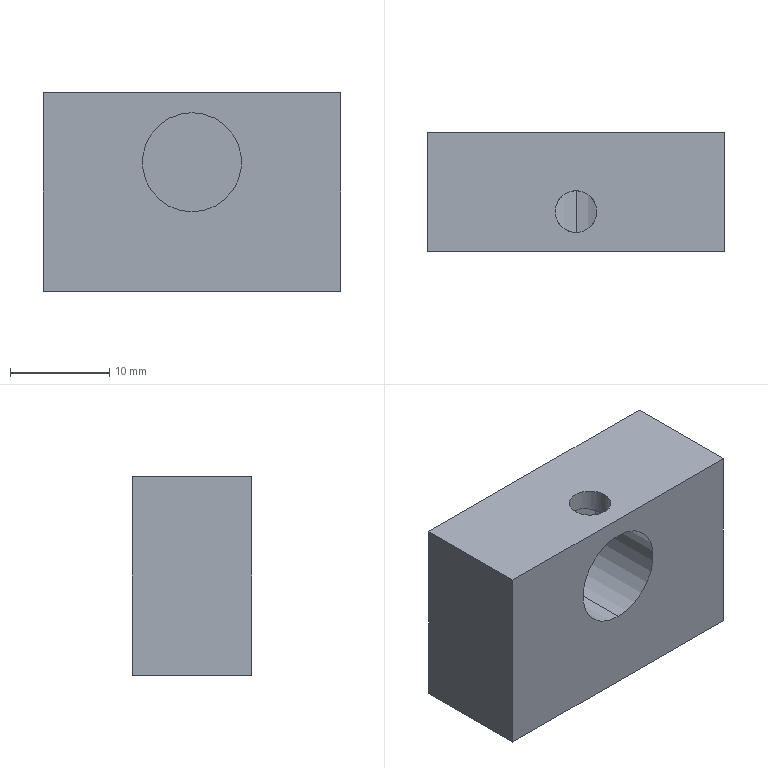Part | STEP file | Magnet seat | 1 solid | 11 faces | box 30 x 12 x 20 mm | volume 6542 mm3 | plane 7 | cylinder 4 | commonest cylinder face diameters 4.2 x2 10 x2
STEP:
#1=CARTESIAN_POINT('',(0.,0.,0.));
#2=DIRECTION('',(0.,0.,1.));
#3=DIRECTION('',(1.,0.,0.));
#4=AXIS2_PLACEMENT_3D('',#1,#2,#3);
#5=CARTESIAN_POINT('',(0.,-4.1,8.));
#6=VERTEX_POINT('',#5);
#7=CARTESIAN_POINT('',(2.1,-2.,7.538));
#8=VERTEX_POINT('',#7);
#9=CARTESIAN_POINT('',(0.,-4.1,8.));
#10=CARTESIAN_POINT('',(0.2769,-4.1,8.));
#11=CARTESIAN_POINT('',(0.5559,-4.044,7.976));
#12=CARTESIAN_POINT('',(0.9357,-3.885,7.913));
#13=CARTESIAN_POINT('',(1.058,-3.819,7.888));
#14=CARTESIAN_POINT('',(1.284,-3.667,7.834));
#15=CARTESIAN_POINT('',(1.389,-3.581,7.804));
#16=CARTESIAN_POINT('',(1.582,-3.388,7.744));
#17=CARTESIAN_POINT('',(1.669,-3.282,7.714));
#18=CARTESIAN_POINT('',(1.82,-3.057,7.658));
#19=CARTESIAN_POINT('',(1.885,-2.937,7.632));
#20=CARTESIAN_POINT('',(1.991,-2.681,7.587));
#21=CARTESIAN_POINT('',(2.031,-2.55,7.569));
#22=CARTESIAN_POINT('',(2.086,-2.28,7.544));
#23=CARTESIAN_POINT('',(2.1,-2.14,7.538));
#24=CARTESIAN_POINT('',(2.1,-2.,7.538));
#25=B_SPLINE_CURVE_WITH_KNOTS('',3,(#9,#10,#11,#12,#13,#14,#15,#16,#17,#18,#19,#20,#21,#22,#23,#24),.UNSPECIFIED.,.F.,.F.,(4,2,2,2,2,2,2,4),(0.009962,0.01079,0.01121,0.01162,0.01204,0.01245,0.01287,0.01328),.UNSPECIFIED.);
#26=CARTESIAN_POINT('',(0.,-2.,10.));
#27=DIRECTION('',(0.,0.,1.));
#28=DIRECTION('',(1.,0.,0.));
#29=AXIS2_PLACEMENT_3D('',#26,#27,#28);
#30=CYLINDRICAL_SURFACE('',#29,2.1);
#31=CARTESIAN_POINT('',(4.712,-2.));
#32=CARTESIAN_POINT('',(4.724,-2.));
#33=CARTESIAN_POINT('',(4.748,-2.));
#34=CARTESIAN_POINT('',(4.784,-2.002));
#35=CARTESIAN_POINT('',(4.82,-2.005));
#36=CARTESIAN_POINT('',(4.857,-2.009));
#37=CARTESIAN_POINT('',(4.893,-2.014));
#38=CARTESIAN_POINT('',(4.929,-2.02));
#39=CARTESIAN_POINT('',(4.965,-2.028));
#40=CARTESIAN_POINT('',(5.001,-2.036));
#41=CARTESIAN_POINT('',(5.036,-2.045));
#42=CARTESIAN_POINT('',(5.072,-2.055));
#43=CARTESIAN_POINT('',(5.108,-2.066));
#44=CARTESIAN_POINT('',(5.144,-2.078));
#45=CARTESIAN_POINT('',(5.179,-2.09));
#46=CARTESIAN_POINT('',(5.215,-2.103));
#47=CARTESIAN_POINT('',(5.251,-2.117));
#48=CARTESIAN_POINT('',(5.286,-2.132));
#49=CARTESIAN_POINT('',(5.322,-2.147));
#50=CARTESIAN_POINT('',(5.357,-2.162));
#51=CARTESIAN_POINT('',(5.392,-2.177));
#52=CARTESIAN_POINT('',(5.428,-2.193));
#53=CARTESIAN_POINT('',(5.463,-2.209));
#54=CARTESIAN_POINT('',(5.498,-2.226));
#55=CARTESIAN_POINT('',(5.534,-2.242));
#56=CARTESIAN_POINT('',(5.569,-2.258));
#57=CARTESIAN_POINT('',(5.604,-2.275));
#58=CARTESIAN_POINT('',(5.64,-2.291));
#59=CARTESIAN_POINT('',(5.675,-2.306));
#60=CARTESIAN_POINT('',(5.71,-2.322));
#61=CARTESIAN_POINT('',(5.745,-2.337));
#62=CARTESIAN_POINT('',(5.781,-2.351));
#63=CARTESIAN_POINT('',(5.816,-2.365));
#64=CARTESIAN_POINT('',(5.852,-2.378));
#65=CARTESIAN_POINT('',(5.888,-2.391));
#66=CARTESIAN_POINT('',(5.924,-2.403));
#67=CARTESIAN_POINT('',(5.959,-2.414));
#68=CARTESIAN_POINT('',(5.995,-2.423));
#69=CARTESIAN_POINT('',(6.031,-2.432));
#70=CARTESIAN_POINT('',(6.066,-2.44));
#71=CARTESIAN_POINT('',(6.102,-2.447));
#72=CARTESIAN_POINT('',(6.138,-2.452));
#73=CARTESIAN_POINT('',(6.174,-2.457));
#74=CARTESIAN_POINT('',(6.21,-2.46));
#75=CARTESIAN_POINT('',(6.247,-2.462));
#76=CARTESIAN_POINT('',(6.271,-2.462));
#77=CARTESIAN_POINT('',(6.283,-2.462));
#78=B_SPLINE_CURVE_WITH_KNOTS('',3,(#31,#32,#33,#34,#35,#36,#37,#38,#39,#40,#41,#42,#43,#44,#45,#46,#47,#48,#49,#50,#51,#52,#53,#54,#55,#56,#57,#58,#59,#60,#61,#62,#63,#64,#65,#66,#67,#68,#69,#70,#71,#72,#73,#74,#75,#76,#77),.UNSPECIFIED.,.F.,.F.,(4,1,1,1,1,1,1,1,1,1,1,1,1,1,1,1,1,1,1,1,1,1,1,1,1,1,1,1,1,1,1,1,1,1,1,1,1,1,1,1,1,1,1,1,4),(0.009962,0.01004,0.01011,0.01019,0.01026,0.01034,0.01041,0.01049,0.01057,0.01064,0.01072,0.01079,0.01087,0.01094,0.01102,0.01109,0.01117,0.01124,0.01132,0.0114,0.01147,0.01155,0.01162,0.0117,0.01177,0.01185,0.01192,0.012,0.01207,0.01215,0.01222,0.0123,0.01238,0.01245,0.01253,0.0126,0.01268,0.01275,0.01283,0.0129,0.01298,0.01305,0.01313,0.01321,0.01328),.QUASI_UNIFORM_KNOTS.);
#79=(GEOMETRIC_REPRESENTATION_CONTEXT(2)PARAMETRIC_REPRESENTATION_CONTEXT()REPRESENTATION_CONTEXT('',''));
#80=DEFINITIONAL_REPRESENTATION('',(#78),#79);
#81=PCURVE('',#30,#80);
#82=CARTESIAN_POINT('',(0.,2.,3.));
#83=DIRECTION('',(0.,-1.,0.));
#84=DIRECTION('',(0.,0.,-1.));
#85=AXIS2_PLACEMENT_3D('',#82,#83,#84);
#86=CYLINDRICAL_SURFACE('',#85,5.);
#87=CARTESIAN_POINT('',(3.142,6.1));
#88=CARTESIAN_POINT('',(3.137,6.1));
#89=CARTESIAN_POINT('',(3.126,6.099));
#90=CARTESIAN_POINT('',(3.111,6.095));
#91=CARTESIAN_POINT('',(3.096,6.088));
#92=CARTESIAN_POINT('',(3.081,6.078));
#93=CARTESIAN_POINT('',(3.066,6.066));
#94=CARTESIAN_POINT('',(3.051,6.051));
#95=CARTESIAN_POINT('',(3.037,6.034));
#96=CARTESIAN_POINT('',(3.022,6.014));
#97=CARTESIAN_POINT('',(3.007,5.991));
#98=CARTESIAN_POINT('',(2.993,5.966));
#99=CARTESIAN_POINT('',(2.979,5.938));
#100=CARTESIAN_POINT('',(2.965,5.908));
#101=CARTESIAN_POINT('',(2.951,5.876));
#102=CARTESIAN_POINT('',(2.938,5.841));
#103=CARTESIAN_POINT('',(2.924,5.803));
#104=CARTESIAN_POINT('',(2.911,5.764));
#105=CARTESIAN_POINT('',(2.899,5.722));
#106=CARTESIAN_POINT('',(2.886,5.679));
#107=CARTESIAN_POINT('',(2.874,5.633));
#108=CARTESIAN_POINT('',(2.863,5.586));
#109=CARTESIAN_POINT('',(2.851,5.536));
#110=CARTESIAN_POINT('',(2.84,5.485));
#111=CARTESIAN_POINT('',(2.829,5.431));
#112=CARTESIAN_POINT('',(2.819,5.376));
#113=CARTESIAN_POINT('',(2.809,5.319));
#114=CARTESIAN_POINT('',(2.799,5.26));
#115=CARTESIAN_POINT('',(2.79,5.2));
#116=CARTESIAN_POINT('',(2.781,5.139));
#117=CARTESIAN_POINT('',(2.772,5.076));
#118=CARTESIAN_POINT('',(2.765,5.012));
#119=CARTESIAN_POINT('',(2.757,4.946));
#120=CARTESIAN_POINT('',(2.75,4.878));
#121=CARTESIAN_POINT('',(2.744,4.809));
#122=CARTESIAN_POINT('',(2.737,4.739));
#123=CARTESIAN_POINT('',(2.732,4.668));
#124=CARTESIAN_POINT('',(2.727,4.597));
#125=CARTESIAN_POINT('',(2.723,4.525));
#126=CARTESIAN_POINT('',(2.719,4.452));
#127=CARTESIAN_POINT('',(2.716,4.378));
#128=CARTESIAN_POINT('',(2.713,4.304));
#129=CARTESIAN_POINT('',(2.711,4.229));
#130=CARTESIAN_POINT('',(2.709,4.153));
#131=CARTESIAN_POINT('',(2.708,4.077));
#132=CARTESIAN_POINT('',(2.708,4.026));
#133=CARTESIAN_POINT('',(2.708,4.));
#134=B_SPLINE_CURVE_WITH_KNOTS('',3,(#87,#88,#89,#90,#91,#92,#93,#94,#95,#96,#97,#98,#99,#100,#101,#102,#103,#104,#105,#106,#107,#108,#109,#110,#111,#112,#113,#114,#115,#116,#117,#118,#119,#120,#121,#122,#123,#124,#125,#126,#127,#128,#129,#130,#131,#132,#133),.UNSPECIFIED.,.F.,.F.,(4,1,1,1,1,1,1,1,1,1,1,1,1,1,1,1,1,1,1,1,1,1,1,1,1,1,1,1,1,1,1,1,1,1,1,1,1,1,1,1,1,1,1,1,4),(0.009962,0.01004,0.01011,0.01019,0.01026,0.01034,0.01041,0.01049,0.01057,0.01064,0.01072,0.01079,0.01087,0.01094,0.01102,0.01109,0.01117,0.01124,0.01132,0.0114,0.01147,0.01155,0.01162,0.0117,0.01177,0.01185,0.01192,0.012,0.01207,0.01215,0.01222,0.0123,0.01238,0.01245,0.01253,0.0126,0.01268,0.01275,0.01283,0.0129,0.01298,0.01305,0.01313,0.01321,0.01328),.QUASI_UNIFORM_KNOTS.);
#135=(GEOMETRIC_REPRESENTATION_CONTEXT(2)PARAMETRIC_REPRESENTATION_CONTEXT()REPRESENTATION_CONTEXT('',''));
#136=DEFINITIONAL_REPRESENTATION('',(#134),#135);
#137=PCURVE('',#86,#136);
#138=SURFACE_CURVE('',#25,(#81,#137),.PCURVE_S1.);
#139=EDGE_CURVE('',#6,#8,#138,.T.);
#140=ORIENTED_EDGE('',*,*,#139,.T.);
#141=CARTESIAN_POINT('',(2.1,-2.,10.));
#142=VERTEX_POINT('',#141);
#143=CARTESIAN_POINT('',(2.1,-2.,10.));
#144=DIRECTION('',(0.,0.,1.));
#145=VECTOR('',#144,1.);
#146=LINE('',#143,#145);
#147=CARTESIAN_POINT('',(6.283,0.));
#148=DIRECTION('',(0.,1.));
#149=VECTOR('',#148,1.);
#150=LINE('',#147,#149);
#151=(GEOMETRIC_REPRESENTATION_CONTEXT(2)PARAMETRIC_REPRESENTATION_CONTEXT()REPRESENTATION_CONTEXT('',''));
#152=DEFINITIONAL_REPRESENTATION('',(#150),#151);
#153=PCURVE('',#30,#152);
#154=CARTESIAN_POINT('',(0.,-2.,10.));
#155=DIRECTION('',(0.,0.,1.));
#156=DIRECTION('',(1.,0.,0.));
#157=AXIS2_PLACEMENT_3D('',#154,#155,#156);
#158=CYLINDRICAL_SURFACE('',#157,2.1);
#159=CARTESIAN_POINT('',(0.,0.));
#160=DIRECTION('',(0.,1.));
#161=VECTOR('',#160,1.);
#162=LINE('',#159,#161);
#163=(GEOMETRIC_REPRESENTATION_CONTEXT(2)PARAMETRIC_REPRESENTATION_CONTEXT()REPRESENTATION_CONTEXT('',''));
#164=DEFINITIONAL_REPRESENTATION('',(#162),#163);
#165=PCURVE('',#158,#164);
#166=SURFACE_CURVE('',#146,(#153,#165),.PCURVE_S1.);
#167=EDGE_CURVE('',#8,#142,#166,.T.);
#168=ORIENTED_EDGE('',*,*,#167,.T.);
#169=CARTESIAN_POINT('',(-2.1,-2.,10.));
#170=VERTEX_POINT('',#169);
#171=CARTESIAN_POINT('',(0.,-2.,10.));
#172=DIRECTION('',(0.,0.,1.));
#173=DIRECTION('',(1.,0.,0.));
#174=AXIS2_PLACEMENT_3D('',#171,#172,#173);
#175=CIRCLE('',#174,2.1);
#176=CARTESIAN_POINT('',(0.,0.));
#177=DIRECTION('',(1.,0.));
#178=VECTOR('',#177,1.);
#179=LINE('',#176,#178);
#180=(GEOMETRIC_REPRESENTATION_CONTEXT(2)PARAMETRIC_REPRESENTATION_CONTEXT()REPRESENTATION_CONTEXT('',''));
#181=DEFINITIONAL_REPRESENTATION('',(#179),#180);
#182=PCURVE('',#30,#181);
#183=CARTESIAN_POINT('',(0.,0.,10.));
#184=DIRECTION('',(0.,0.,-1.));
#185=DIRECTION('',(-1.,0.,0.));
#186=AXIS2_PLACEMENT_3D('',#183,#184,#185);
#187=PLANE('',#186);
#188=CARTESIAN_POINT('',(-2.1,-2.));
#189=CARTESIAN_POINT('',(-2.1,1.637));
#190=CARTESIAN_POINT('',(1.05,-0.1813));
#191=CARTESIAN_POINT('',(4.2,-2.));
#192=CARTESIAN_POINT('',(1.05,-3.819));
#193=CARTESIAN_POINT('',(-2.1,-5.637));
#194=CARTESIAN_POINT('',(-2.1,-2.));
#195=(BOUNDED_CURVE()B_SPLINE_CURVE(2,(#188,#189,#190,#191,#192,#193,#194),.UNSPECIFIED.,.T.,.F.)B_SPLINE_CURVE_WITH_KNOTS((1,2,2,2,2,1),(-2.094,0.,2.094,4.189,6.283,8.378),.UNSPECIFIED.)CURVE()GEOMETRIC_REPRESENTATION_ITEM()RATIONAL_B_SPLINE_CURVE((1.,0.5,1.,0.5,1.,0.5,1.))REPRESENTATION_ITEM(''));
#196=(GEOMETRIC_REPRESENTATION_CONTEXT(2)PARAMETRIC_REPRESENTATION_CONTEXT()REPRESENTATION_CONTEXT('',''));
#197=DEFINITIONAL_REPRESENTATION('',(#195),#196);
#198=PCURVE('',#187,#197);
#199=SURFACE_CURVE('',#175,(#182,#198),.PCURVE_S1.);
#200=EDGE_CURVE('',#170,#142,#199,.T.);
#201=ORIENTED_EDGE('',*,*,#200,.F.);
#202=CARTESIAN_POINT('',(-2.1,-2.,7.538));
#203=VERTEX_POINT('',#202);
#204=CARTESIAN_POINT('',(-2.1,-2.,10.));
#205=DIRECTION('',(0.,0.,1.));
#206=VECTOR('',#205,1.);
#207=LINE('',#204,#206);
#208=CARTESIAN_POINT('',(3.142,0.));
#209=DIRECTION('',(0.,1.));
#210=VECTOR('',#209,1.);
#211=LINE('',#208,#210);
#212=(GEOMETRIC_REPRESENTATION_CONTEXT(2)PARAMETRIC_REPRESENTATION_CONTEXT()REPRESENTATION_CONTEXT('',''));
#213=DEFINITIONAL_REPRESENTATION('',(#211),#212);
#214=PCURVE('',#30,#213);
#215=CARTESIAN_POINT('',(3.142,0.));
#216=DIRECTION('',(0.,1.));
#217=VECTOR('',#216,1.);
#218=LINE('',#215,#217);
#219=(GEOMETRIC_REPRESENTATION_CONTEXT(2)PARAMETRIC_REPRESENTATION_CONTEXT()REPRESENTATION_CONTEXT('',''));
#220=DEFINITIONAL_REPRESENTATION('',(#218),#219);
#221=PCURVE('',#158,#220);
#222=SURFACE_CURVE('',#207,(#214,#221),.PCURVE_S1.);
#223=EDGE_CURVE('',#203,#170,#222,.T.);
#224=ORIENTED_EDGE('',*,*,#223,.F.);
#225=CARTESIAN_POINT('',(-2.1,-2.,7.538));
#226=CARTESIAN_POINT('',(-2.1,-2.138,7.538));
#227=CARTESIAN_POINT('',(-2.086,-2.279,7.544));
#228=CARTESIAN_POINT('',(-2.031,-2.551,7.569));
#229=CARTESIAN_POINT('',(-1.991,-2.682,7.587));
#230=CARTESIAN_POINT('',(-1.832,-3.063,7.654));
#231=CARTESIAN_POINT('',(-1.678,-3.292,7.715));
#232=CARTESIAN_POINT('',(-1.388,-3.582,7.805));
#233=CARTESIAN_POINT('',(-1.283,-3.668,7.834));
#234=CARTESIAN_POINT('',(-1.058,-3.819,7.888));
#235=CARTESIAN_POINT('',(-0.9352,-3.885,7.913));
#236=CARTESIAN_POINT('',(-0.6818,-3.991,7.955));
#237=CARTESIAN_POINT('',(-0.5507,-4.031,7.971));
#238=CARTESIAN_POINT('',(-0.2793,-4.086,7.994));
#239=CARTESIAN_POINT('',(-0.1385,-4.1,8.));
#240=CARTESIAN_POINT('',(0.,-4.1,8.));
#241=B_SPLINE_CURVE_WITH_KNOTS('',3,(#225,#226,#227,#228,#229,#230,#231,#232,#233,#234,#235,#236,#237,#238,#239,#240),.UNSPECIFIED.,.F.,.F.,(4,2,2,2,2,2,2,4),(0.006643,0.007058,0.007473,0.008303,0.008718,0.009133,0.009547,0.009962),.UNSPECIFIED.);
#242=CARTESIAN_POINT('',(3.142,-2.462));
#243=CARTESIAN_POINT('',(3.154,-2.462));
#244=CARTESIAN_POINT('',(3.178,-2.462));
#245=CARTESIAN_POINT('',(3.214,-2.46));
#246=CARTESIAN_POINT('',(3.25,-2.457));
#247=CARTESIAN_POINT('',(3.286,-2.452));
#248=CARTESIAN_POINT('',(3.322,-2.447));
#249=CARTESIAN_POINT('',(3.358,-2.44));
#250=CARTESIAN_POINT('',(3.394,-2.432));
#251=CARTESIAN_POINT('',(3.43,-2.423));
#252=CARTESIAN_POINT('',(3.466,-2.414));
#253=CARTESIAN_POINT('',(3.501,-2.403));
#254=CARTESIAN_POINT('',(3.537,-2.391));
#255=CARTESIAN_POINT('',(3.573,-2.378));
#256=CARTESIAN_POINT('',(3.608,-2.365));
#257=CARTESIAN_POINT('',(3.644,-2.351));
#258=CARTESIAN_POINT('',(3.679,-2.337));
#259=CARTESIAN_POINT('',(3.715,-2.322));
#260=CARTESIAN_POINT('',(3.75,-2.306));
#261=CARTESIAN_POINT('',(3.786,-2.29));
#262=CARTESIAN_POINT('',(3.821,-2.274));
#263=CARTESIAN_POINT('',(3.856,-2.258));
#264=CARTESIAN_POINT('',(3.892,-2.242));
#265=CARTESIAN_POINT('',(3.927,-2.225));
#266=CARTESIAN_POINT('',(3.963,-2.209));
#267=CARTESIAN_POINT('',(3.998,-2.193));
#268=CARTESIAN_POINT('',(4.033,-2.177));
#269=CARTESIAN_POINT('',(4.068,-2.162));
#270=CARTESIAN_POINT('',(4.104,-2.146));
#271=CARTESIAN_POINT('',(4.139,-2.132));
#272=CARTESIAN_POINT('',(4.174,-2.117));
#273=CARTESIAN_POINT('',(4.21,-2.103));
#274=CARTESIAN_POINT('',(4.246,-2.09));
#275=CARTESIAN_POINT('',(4.281,-2.077));
#276=CARTESIAN_POINT('',(4.317,-2.066));
#277=CARTESIAN_POINT('',(4.353,-2.055));
#278=CARTESIAN_POINT('',(4.388,-2.045));
#279=CARTESIAN_POINT('',(4.424,-2.036));
#280=CARTESIAN_POINT('',(4.46,-2.027));
#281=CARTESIAN_POINT('',(4.495,-2.02));
#282=CARTESIAN_POINT('',(4.531,-2.014));
#283=CARTESIAN_POINT('',(4.568,-2.009));
#284=CARTESIAN_POINT('',(4.604,-2.005));
#285=CARTESIAN_POINT('',(4.64,-2.002));
#286=CARTESIAN_POINT('',(4.676,-2.));
#287=CARTESIAN_POINT('',(4.7,-2.));
#288=CARTESIAN_POINT('',(4.712,-2.));
#289=B_SPLINE_CURVE_WITH_KNOTS('',3,(#242,#243,#244,#245,#246,#247,#248,#249,#250,#251,#252,#253,#254,#255,#256,#257,#258,#259,#260,#261,#262,#263,#264,#265,#266,#267,#268,#269,#270,#271,#272,#273,#274,#275,#276,#277,#278,#279,#280,#281,#282,#283,#284,#285,#286,#287,#288),.UNSPECIFIED.,.F.,.F.,(4,1,1,1,1,1,1,1,1,1,1,1,1,1,1,1,1,1,1,1,1,1,1,1,1,1,1,1,1,1,1,1,1,1,1,1,1,1,1,1,1,1,1,1,4),(0.006643,0.006719,0.006794,0.006869,0.006945,0.00702,0.007096,0.007171,0.007247,0.007322,0.007397,0.007473,0.007548,0.007624,0.007699,0.007775,0.00785,0.007926,0.008001,0.008076,0.008152,0.008227,0.008303,0.008378,0.008454,0.008529,0.008604,0.00868,0.008755,0.008831,0.008906,0.008982,0.009057,0.009133,0.009208,0.009283,0.009359,0.009434,0.00951,0.009585,0.009661,0.009736,0.009811,0.009887,0.009962),.QUASI_UNIFORM_KNOTS.);
#290=(GEOMETRIC_REPRESENTATION_CONTEXT(2)PARAMETRIC_REPRESENTATION_CONTEXT()REPRESENTATION_CONTEXT('',''));
#291=DEFINITIONAL_REPRESENTATION('',(#289),#290);
#292=PCURVE('',#30,#291);
#293=CARTESIAN_POINT('',(0.,2.,3.));
#294=DIRECTION('',(0.,-1.,0.));
#295=DIRECTION('',(0.,0.,-1.));
#296=AXIS2_PLACEMENT_3D('',#293,#294,#295);
#297=CYLINDRICAL_SURFACE('',#296,5.);
#298=CARTESIAN_POINT('',(3.575,4.));
#299=CARTESIAN_POINT('',(3.575,4.025));
#300=CARTESIAN_POINT('',(3.575,4.076));
#301=CARTESIAN_POINT('',(3.574,4.151));
#302=CARTESIAN_POINT('',(3.572,4.227));
#303=CARTESIAN_POINT('',(3.57,4.303));
#304=CARTESIAN_POINT('',(3.568,4.378));
#305=CARTESIAN_POINT('',(3.564,4.452));
#306=CARTESIAN_POINT('',(3.56,4.525));
#307=CARTESIAN_POINT('',(3.556,4.597));
#308=CARTESIAN_POINT('',(3.551,4.669));
#309=CARTESIAN_POINT('',(3.546,4.739));
#310=CARTESIAN_POINT('',(3.54,4.809));
#311=CARTESIAN_POINT('',(3.533,4.878));
#312=CARTESIAN_POINT('',(3.526,4.945));
#313=CARTESIAN_POINT('',(3.519,5.011));
#314=CARTESIAN_POINT('',(3.511,5.076));
#315=CARTESIAN_POINT('',(3.502,5.139));
#316=CARTESIAN_POINT('',(3.493,5.201));
#317=CARTESIAN_POINT('',(3.484,5.261));
#318=CARTESIAN_POINT('',(3.474,5.32));
#319=CARTESIAN_POINT('',(3.464,5.377));
#320=CARTESIAN_POINT('',(3.454,5.432));
#321=CARTESIAN_POINT('',(3.443,5.486));
#322=CARTESIAN_POINT('',(3.432,5.537));
#323=CARTESIAN_POINT('',(3.42,5.587));
#324=CARTESIAN_POINT('',(3.409,5.634));
#325=CARTESIAN_POINT('',(3.397,5.68));
#326=CARTESIAN_POINT('',(3.384,5.723));
#327=CARTESIAN_POINT('',(3.372,5.764));
#328=CARTESIAN_POINT('',(3.359,5.804));
#329=CARTESIAN_POINT('',(3.345,5.841));
#330=CARTESIAN_POINT('',(3.332,5.876));
#331=CARTESIAN_POINT('',(3.318,5.908));
#332=CARTESIAN_POINT('',(3.304,5.939));
#333=CARTESIAN_POINT('',(3.29,5.966));
#334=CARTESIAN_POINT('',(3.276,5.991));
#335=CARTESIAN_POINT('',(3.261,6.014));
#336=CARTESIAN_POINT('',(3.247,6.034));
#337=CARTESIAN_POINT('',(3.232,6.051));
#338=CARTESIAN_POINT('',(3.217,6.066));
#339=CARTESIAN_POINT('',(3.202,6.078));
#340=CARTESIAN_POINT('',(3.187,6.088));
#341=CARTESIAN_POINT('',(3.172,6.095));
#342=CARTESIAN_POINT('',(3.157,6.099));
#343=CARTESIAN_POINT('',(3.147,6.1));
#344=CARTESIAN_POINT('',(3.142,6.1));
#345=B_SPLINE_CURVE_WITH_KNOTS('',3,(#298,#299,#300,#301,#302,#303,#304,#305,#306,#307,#308,#309,#310,#311,#312,#313,#314,#315,#316,#317,#318,#319,#320,#321,#322,#323,#324,#325,#326,#327,#328,#329,#330,#331,#332,#333,#334,#335,#336,#337,#338,#339,#340,#341,#342,#343,#344),.UNSPECIFIED.,.F.,.F.,(4,1,1,1,1,1,1,1,1,1,1,1,1,1,1,1,1,1,1,1,1,1,1,1,1,1,1,1,1,1,1,1,1,1,1,1,1,1,1,1,1,1,1,1,4),(0.006643,0.006719,0.006794,0.006869,0.006945,0.00702,0.007096,0.007171,0.007247,0.007322,0.007397,0.007473,0.007548,0.007624,0.007699,0.007775,0.00785,0.007926,0.008001,0.008076,0.008152,0.008227,0.008303,0.008378,0.008454,0.008529,0.008604,0.00868,0.008755,0.008831,0.008906,0.008982,0.009057,0.009133,0.009208,0.009283,0.009359,0.009434,0.00951,0.009585,0.009661,0.009736,0.009811,0.009887,0.009962),.QUASI_UNIFORM_KNOTS.);
#346=(GEOMETRIC_REPRESENTATION_CONTEXT(2)PARAMETRIC_REPRESENTATION_CONTEXT()REPRESENTATION_CONTEXT('',''));
#347=DEFINITIONAL_REPRESENTATION('',(#345),#346);
#348=PCURVE('',#297,#347);
#349=SURFACE_CURVE('',#241,(#292,#348),.PCURVE_S1.);
#350=EDGE_CURVE('',#203,#6,#349,.T.);
#351=ORIENTED_EDGE('',*,*,#350,.T.);
#352=EDGE_LOOP('',(#140,#168,#201,#224,#351));
#353=FACE_BOUND('',#352,.F.);
#354=ADVANCED_FACE('',(#353),#30,.F.);
#355=CARTESIAN_POINT('',(0.,2.,-2.));
#356=VERTEX_POINT('',#355);
#357=CARTESIAN_POINT('',(0.,-6.,-2.));
#358=VERTEX_POINT('',#357);
#359=CARTESIAN_POINT('',(0.,2.,-2.));
#360=DIRECTION('',(0.,-1.,0.));
#361=VECTOR('',#360,1.);
#362=LINE('',#359,#361);
#363=CARTESIAN_POINT('',(6.283,0.));
#364=DIRECTION('',(0.,1.));
#365=VECTOR('',#364,1.);
#366=LINE('',#363,#365);
#367=(GEOMETRIC_REPRESENTATION_CONTEXT(2)PARAMETRIC_REPRESENTATION_CONTEXT()REPRESENTATION_CONTEXT('',''));
#368=DEFINITIONAL_REPRESENTATION('',(#366),#367);
#369=PCURVE('',#297,#368);
#370=CARTESIAN_POINT('',(0.,0.));
#371=DIRECTION('',(0.,1.));
#372=VECTOR('',#371,1.);
#373=LINE('',#370,#372);
#374=(GEOMETRIC_REPRESENTATION_CONTEXT(2)PARAMETRIC_REPRESENTATION_CONTEXT()REPRESENTATION_CONTEXT('',''));
#375=DEFINITIONAL_REPRESENTATION('',(#373),#374);
#376=PCURVE('',#86,#375);
#377=SURFACE_CURVE('',#362,(#369,#376),.PCURVE_S1.);
#378=EDGE_CURVE('',#356,#358,#377,.T.);
#379=ORIENTED_EDGE('',*,*,#378,.T.);
#380=CARTESIAN_POINT('',(0.,-6.,8.));
#381=VERTEX_POINT('',#380);
#382=CARTESIAN_POINT('',(0.,-6.,3.));
#383=DIRECTION('',(0.,-1.,0.));
#384=DIRECTION('',(0.,0.,-1.));
#385=AXIS2_PLACEMENT_3D('',#382,#383,#384);
#386=CIRCLE('',#385,5.);
#387=CARTESIAN_POINT('',(0.,8.));
#388=DIRECTION('',(1.,0.));
#389=VECTOR('',#388,1.);
#390=LINE('',#387,#389);
#391=(GEOMETRIC_REPRESENTATION_CONTEXT(2)PARAMETRIC_REPRESENTATION_CONTEXT()REPRESENTATION_CONTEXT('',''));
#392=DEFINITIONAL_REPRESENTATION('',(#390),#391);
#393=PCURVE('',#297,#392);
#394=CARTESIAN_POINT('',(-15.,-6.,10.));
#395=DIRECTION('',(0.,1.,0.));
#396=DIRECTION('',(0.,0.,1.));
#397=AXIS2_PLACEMENT_3D('',#394,#395,#396);
#398=PLANE('',#397);
#399=CARTESIAN_POINT('',(-12.,15.));
#400=CARTESIAN_POINT('',(-12.,23.66));
#401=CARTESIAN_POINT('',(-4.5,19.33));
#402=CARTESIAN_POINT('',(3.,15.));
#403=CARTESIAN_POINT('',(-4.5,10.67));
#404=CARTESIAN_POINT('',(-12.,6.34));
#405=CARTESIAN_POINT('',(-12.,15.));
#406=(BOUNDED_CURVE()B_SPLINE_CURVE(2,(#399,#400,#401,#402,#403,#404,#405),.UNSPECIFIED.,.T.,.F.)B_SPLINE_CURVE_WITH_KNOTS((1,2,2,2,2,1),(-2.094,0.,2.094,4.189,6.283,8.378),.UNSPECIFIED.)CURVE()GEOMETRIC_REPRESENTATION_ITEM()RATIONAL_B_SPLINE_CURVE((1.,0.5,1.,0.5,1.,0.5,1.))REPRESENTATION_ITEM(''));
#407=(GEOMETRIC_REPRESENTATION_CONTEXT(2)PARAMETRIC_REPRESENTATION_CONTEXT()REPRESENTATION_CONTEXT('',''));
#408=DEFINITIONAL_REPRESENTATION('',(#406),#407);
#409=PCURVE('',#398,#408);
#410=SURFACE_CURVE('',#386,(#393,#409),.PCURVE_S1.);
#411=EDGE_CURVE('',#381,#358,#410,.T.);
#412=ORIENTED_EDGE('',*,*,#411,.F.);
#413=CARTESIAN_POINT('',(0.,2.,8.));
#414=DIRECTION('',(0.,-1.,0.));
#415=VECTOR('',#414,1.);
#416=LINE('',#413,#415);
#417=CARTESIAN_POINT('',(3.142,0.));
#418=DIRECTION('',(0.,1.));
#419=VECTOR('',#418,1.);
#420=LINE('',#417,#419);
#421=(GEOMETRIC_REPRESENTATION_CONTEXT(2)PARAMETRIC_REPRESENTATION_CONTEXT()REPRESENTATION_CONTEXT('',''));
#422=DEFINITIONAL_REPRESENTATION('',(#420),#421);
#423=PCURVE('',#297,#422);
#424=CARTESIAN_POINT('',(3.142,0.));
#425=DIRECTION('',(0.,1.));
#426=VECTOR('',#425,1.);
#427=LINE('',#424,#426);
#428=(GEOMETRIC_REPRESENTATION_CONTEXT(2)PARAMETRIC_REPRESENTATION_CONTEXT()REPRESENTATION_CONTEXT('',''));
#429=DEFINITIONAL_REPRESENTATION('',(#427),#428);
#430=PCURVE('',#86,#429);
#431=SURFACE_CURVE('',#416,(#423,#430),.PCURVE_S1.);
#432=EDGE_CURVE('',#6,#381,#431,.T.);
#433=ORIENTED_EDGE('',*,*,#432,.F.);
#434=ORIENTED_EDGE('',*,*,#350,.F.);
#435=CARTESIAN_POINT('',(0.,0.1,8.));
#436=VERTEX_POINT('',#435);
#437=CARTESIAN_POINT('',(0.,0.1,8.));
#438=CARTESIAN_POINT('',(-0.1389,0.1,8.));
#439=CARTESIAN_POINT('',(-0.2797,0.08587,7.994));
#440=CARTESIAN_POINT('',(-0.5505,0.03126,7.971));
#441=CARTESIAN_POINT('',(-0.6827,-0.009253,7.955));
#442=CARTESIAN_POINT('',(-0.9385,-0.1163,7.913));
#443=CARTESIAN_POINT('',(-1.059,-0.1813,7.888));
#444=CARTESIAN_POINT('',(-1.285,-0.3331,7.834));
#445=CARTESIAN_POINT('',(-1.391,-0.421,7.804));
#446=CARTESIAN_POINT('',(-1.583,-0.6132,7.744));
#447=CARTESIAN_POINT('',(-1.669,-0.7177,7.714));
#448=CARTESIAN_POINT('',(-1.821,-0.9444,7.658));
#449=CARTESIAN_POINT('',(-1.886,-1.066,7.631));
#450=CARTESIAN_POINT('',(-2.043,-1.444,7.565));
#451=CARTESIAN_POINT('',(-2.1,-1.723,7.538));
#452=CARTESIAN_POINT('',(-2.1,-2.,7.538));
#453=B_SPLINE_CURVE_WITH_KNOTS('',3,(#437,#438,#439,#440,#441,#442,#443,#444,#445,#446,#447,#448,#449,#450,#451,#452),.UNSPECIFIED.,.F.,.F.,(4,2,2,2,2,2,2,4),(0.003323,0.003738,0.004153,0.004568,0.004983,0.005398,0.005813,0.006643),.UNSPECIFIED.);
#454=CARTESIAN_POINT('',(3.142,1.9));
#455=CARTESIAN_POINT('',(3.147,1.9));
#456=CARTESIAN_POINT('',(3.157,1.901));
#457=CARTESIAN_POINT('',(3.172,1.905));
#458=CARTESIAN_POINT('',(3.187,1.912));
#459=CARTESIAN_POINT('',(3.202,1.922));
#460=CARTESIAN_POINT('',(3.217,1.934));
#461=CARTESIAN_POINT('',(3.232,1.949));
#462=CARTESIAN_POINT('',(3.247,1.966));
#463=CARTESIAN_POINT('',(3.261,1.986));
#464=CARTESIAN_POINT('',(3.276,2.009));
#465=CARTESIAN_POINT('',(3.29,2.034));
#466=CARTESIAN_POINT('',(3.304,2.062));
#467=CARTESIAN_POINT('',(3.318,2.093));
#468=CARTESIAN_POINT('',(3.332,2.125));
#469=CARTESIAN_POINT('',(3.346,2.16));
#470=CARTESIAN_POINT('',(3.359,2.197));
#471=CARTESIAN_POINT('',(3.372,2.236));
#472=CARTESIAN_POINT('',(3.384,2.278));
#473=CARTESIAN_POINT('',(3.397,2.322));
#474=CARTESIAN_POINT('',(3.409,2.367));
#475=CARTESIAN_POINT('',(3.421,2.415));
#476=CARTESIAN_POINT('',(3.432,2.465));
#477=CARTESIAN_POINT('',(3.444,2.517));
#478=CARTESIAN_POINT('',(3.454,2.57));
#479=CARTESIAN_POINT('',(3.465,2.625));
#480=CARTESIAN_POINT('',(3.475,2.682));
#481=CARTESIAN_POINT('',(3.484,2.74));
#482=CARTESIAN_POINT('',(3.494,2.8));
#483=CARTESIAN_POINT('',(3.502,2.862));
#484=CARTESIAN_POINT('',(3.511,2.925));
#485=CARTESIAN_POINT('',(3.519,2.99));
#486=CARTESIAN_POINT('',(3.526,3.056));
#487=CARTESIAN_POINT('',(3.533,3.124));
#488=CARTESIAN_POINT('',(3.54,3.192));
#489=CARTESIAN_POINT('',(3.546,3.261));
#490=CARTESIAN_POINT('',(3.551,3.332));
#491=CARTESIAN_POINT('',(3.556,3.404));
#492=CARTESIAN_POINT('',(3.56,3.476));
#493=CARTESIAN_POINT('',(3.564,3.55));
#494=CARTESIAN_POINT('',(3.568,3.624));
#495=CARTESIAN_POINT('',(3.57,3.699));
#496=CARTESIAN_POINT('',(3.572,3.774));
#497=CARTESIAN_POINT('',(3.574,3.849));
#498=CARTESIAN_POINT('',(3.575,3.925));
#499=CARTESIAN_POINT('',(3.575,3.975));
#500=CARTESIAN_POINT('',(3.575,4.));
#501=B_SPLINE_CURVE_WITH_KNOTS('',3,(#454,#455,#456,#457,#458,#459,#460,#461,#462,#463,#464,#465,#466,#467,#468,#469,#470,#471,#472,#473,#474,#475,#476,#477,#478,#479,#480,#481,#482,#483,#484,#485,#486,#487,#488,#489,#490,#491,#492,#493,#494,#495,#496,#497,#498,#499,#500),.UNSPECIFIED.,.F.,.F.,(4,1,1,1,1,1,1,1,1,1,1,1,1,1,1,1,1,1,1,1,1,1,1,1,1,1,1,1,1,1,1,1,1,1,1,1,1,1,1,1,1,1,1,1,4),(0.003323,0.003398,0.003474,0.003549,0.003625,0.0037,0.003775,0.003851,0.003926,0.004002,0.004077,0.004153,0.004228,0.004304,0.004379,0.004455,0.00453,0.004606,0.004681,0.004757,0.004832,0.004907,0.004983,0.005058,0.005134,0.005209,0.005285,0.00536,0.005436,0.005511,0.005587,0.005662,0.005738,0.005813,0.005888,0.005964,0.006039,0.006115,0.00619,0.006266,0.006341,0.006417,0.006492,0.006568,0.006643),.QUASI_UNIFORM_KNOTS.);
#502=(GEOMETRIC_REPRESENTATION_CONTEXT(2)PARAMETRIC_REPRESENTATION_CONTEXT()REPRESENTATION_CONTEXT('',''));
#503=DEFINITIONAL_REPRESENTATION('',(#501),#502);
#504=PCURVE('',#297,#503);
#505=CARTESIAN_POINT('',(1.571,-2.));
#506=CARTESIAN_POINT('',(1.583,-2.));
#507=CARTESIAN_POINT('',(1.607,-2.));
#508=CARTESIAN_POINT('',(1.643,-2.002));
#509=CARTESIAN_POINT('',(1.679,-2.005));
#510=CARTESIAN_POINT('',(1.716,-2.009));
#511=CARTESIAN_POINT('',(1.752,-2.014));
#512=CARTESIAN_POINT('',(1.788,-2.02));
#513=CARTESIAN_POINT('',(1.824,-2.027));
#514=CARTESIAN_POINT('',(1.859,-2.036));
#515=CARTESIAN_POINT('',(1.895,-2.045));
#516=CARTESIAN_POINT('',(1.931,-2.055));
#517=CARTESIAN_POINT('',(1.967,-2.066));
#518=CARTESIAN_POINT('',(2.003,-2.078));
#519=CARTESIAN_POINT('',(2.039,-2.09));
#520=CARTESIAN_POINT('',(2.074,-2.104));
#521=CARTESIAN_POINT('',(2.11,-2.117));
#522=CARTESIAN_POINT('',(2.145,-2.132));
#523=CARTESIAN_POINT('',(2.18,-2.147));
#524=CARTESIAN_POINT('',(2.216,-2.162));
#525=CARTESIAN_POINT('',(2.251,-2.178));
#526=CARTESIAN_POINT('',(2.287,-2.194));
#527=CARTESIAN_POINT('',(2.322,-2.21));
#528=CARTESIAN_POINT('',(2.358,-2.226));
#529=CARTESIAN_POINT('',(2.393,-2.242));
#530=CARTESIAN_POINT('',(2.428,-2.259));
#531=CARTESIAN_POINT('',(2.463,-2.275));
#532=CARTESIAN_POINT('',(2.498,-2.291));
#533=CARTESIAN_POINT('',(2.534,-2.307));
#534=CARTESIAN_POINT('',(2.569,-2.322));
#535=CARTESIAN_POINT('',(2.604,-2.337));
#536=CARTESIAN_POINT('',(2.64,-2.352));
#537=CARTESIAN_POINT('',(2.676,-2.365));
#538=CARTESIAN_POINT('',(2.711,-2.379));
#539=CARTESIAN_POINT('',(2.747,-2.391));
#540=CARTESIAN_POINT('',(2.782,-2.403));
#541=CARTESIAN_POINT('',(2.818,-2.414));
#542=CARTESIAN_POINT('',(2.854,-2.423));
#543=CARTESIAN_POINT('',(2.89,-2.432));
#544=CARTESIAN_POINT('',(2.926,-2.44));
#545=CARTESIAN_POINT('',(2.962,-2.447));
#546=CARTESIAN_POINT('',(2.998,-2.452));
#547=CARTESIAN_POINT('',(3.034,-2.457));
#548=CARTESIAN_POINT('',(3.07,-2.46));
#549=CARTESIAN_POINT('',(3.106,-2.462));
#550=CARTESIAN_POINT('',(3.13,-2.462));
#551=CARTESIAN_POINT('',(3.142,-2.462));
#552=B_SPLINE_CURVE_WITH_KNOTS('',3,(#505,#506,#507,#508,#509,#510,#511,#512,#513,#514,#515,#516,#517,#518,#519,#520,#521,#522,#523,#524,#525,#526,#527,#528,#529,#530,#531,#532,#533,#534,#535,#536,#537,#538,#539,#540,#541,#542,#543,#544,#545,#546,#547,#548,#549,#550,#551),.UNSPECIFIED.,.F.,.F.,(4,1,1,1,1,1,1,1,1,1,1,1,1,1,1,1,1,1,1,1,1,1,1,1,1,1,1,1,1,1,1,1,1,1,1,1,1,1,1,1,1,1,1,1,4),(0.003323,0.003398,0.003474,0.003549,0.003625,0.0037,0.003775,0.003851,0.003926,0.004002,0.004077,0.004153,0.004228,0.004304,0.004379,0.004455,0.00453,0.004606,0.004681,0.004757,0.004832,0.004907,0.004983,0.005058,0.005134,0.005209,0.005285,0.00536,0.005436,0.005511,0.005587,0.005662,0.005738,0.005813,0.005888,0.005964,0.006039,0.006115,0.00619,0.006266,0.006341,0.006417,0.006492,0.006568,0.006643),.QUASI_UNIFORM_KNOTS.);
#553=(GEOMETRIC_REPRESENTATION_CONTEXT(2)PARAMETRIC_REPRESENTATION_CONTEXT()REPRESENTATION_CONTEXT('',''));
#554=DEFINITIONAL_REPRESENTATION('',(#552),#553);
#555=PCURVE('',#158,#554);
#556=SURFACE_CURVE('',#453,(#504,#555),.PCURVE_S1.);
#557=EDGE_CURVE('',#436,#203,#556,.T.);
#558=ORIENTED_EDGE('',*,*,#557,.F.);
#559=CARTESIAN_POINT('',(0.,2.,8.));
#560=VERTEX_POINT('',#559);
#561=CARTESIAN_POINT('',(0.,2.,8.));
#562=DIRECTION('',(0.,-1.,0.));
#563=VECTOR('',#562,1.);
#564=LINE('',#561,#563);
#565=CARTESIAN_POINT('',(3.142,0.));
#566=DIRECTION('',(0.,1.));
#567=VECTOR('',#566,1.);
#568=LINE('',#565,#567);
#569=(GEOMETRIC_REPRESENTATION_CONTEXT(2)PARAMETRIC_REPRESENTATION_CONTEXT()REPRESENTATION_CONTEXT('',''));
#570=DEFINITIONAL_REPRESENTATION('',(#568),#569);
#571=PCURVE('',#297,#570);
#572=CARTESIAN_POINT('',(3.142,0.));
#573=DIRECTION('',(0.,1.));
#574=VECTOR('',#573,1.);
#575=LINE('',#572,#574);
#576=(GEOMETRIC_REPRESENTATION_CONTEXT(2)PARAMETRIC_REPRESENTATION_CONTEXT()REPRESENTATION_CONTEXT('',''));
#577=DEFINITIONAL_REPRESENTATION('',(#575),#576);
#578=PCURVE('',#86,#577);
#579=SURFACE_CURVE('',#564,(#571,#578),.PCURVE_S1.);
#580=EDGE_CURVE('',#560,#436,#579,.T.);
#581=ORIENTED_EDGE('',*,*,#580,.F.);
#582=CARTESIAN_POINT('',(0.,2.,3.));
#583=DIRECTION('',(0.,-1.,0.));
#584=DIRECTION('',(0.,0.,-1.));
#585=AXIS2_PLACEMENT_3D('',#582,#583,#584);
#586=CIRCLE('',#585,5.);
#587=CARTESIAN_POINT('',(0.,0.));
#588=DIRECTION('',(1.,0.));
#589=VECTOR('',#588,1.);
#590=LINE('',#587,#589);
#591=(GEOMETRIC_REPRESENTATION_CONTEXT(2)PARAMETRIC_REPRESENTATION_CONTEXT()REPRESENTATION_CONTEXT('',''));
#592=DEFINITIONAL_REPRESENTATION('',(#590),#591);
#593=PCURVE('',#297,#592);
#594=CARTESIAN_POINT('',(0.,2.,3.));
#595=DIRECTION('',(0.,-1.,0.));
#596=DIRECTION('',(0.,0.,-1.));
#597=AXIS2_PLACEMENT_3D('',#594,#595,#596);
#598=PLANE('',#597);
#599=CARTESIAN_POINT('',(0.,0.));
#600=DIRECTION('',(1.,0.));
#601=AXIS2_PLACEMENT_2D('',#599,#600);
#602=CIRCLE('',#601,5.);
#603=(GEOMETRIC_REPRESENTATION_CONTEXT(2)PARAMETRIC_REPRESENTATION_CONTEXT()REPRESENTATION_CONTEXT('',''));
#604=DEFINITIONAL_REPRESENTATION('',(#602),#603);
#605=PCURVE('',#598,#604);
#606=SURFACE_CURVE('',#586,(#593,#605),.PCURVE_S1.);
#607=EDGE_CURVE('',#560,#356,#606,.T.);
#608=ORIENTED_EDGE('',*,*,#607,.T.);
#609=EDGE_LOOP('',(#379,#412,#433,#434,#558,#581,#608));
#610=FACE_BOUND('',#609,.F.);
#611=ADVANCED_FACE('',(#610),#297,.F.);
#612=CARTESIAN_POINT('',(15.,-6.,-10.));
#613=VERTEX_POINT('',#612);
#614=CARTESIAN_POINT('',(15.,6.,-10.));
#615=VERTEX_POINT('',#614);
#616=CARTESIAN_POINT('',(15.,-6.,-10.));
#617=DIRECTION('',(0.,1.,0.));
#618=VECTOR('',#617,1.);
#619=LINE('',#616,#618);
#620=CARTESIAN_POINT('',(15.,-6.,10.));
#621=DIRECTION('',(-1.,0.,0.));
#622=DIRECTION('',(0.,0.,1.));
#623=AXIS2_PLACEMENT_3D('',#620,#621,#622);
#624=PLANE('',#623);
#625=CARTESIAN_POINT('',(-20.,0.));
#626=DIRECTION('',(0.,1.));
#627=VECTOR('',#626,1.);
#628=LINE('',#625,#627);
#629=(GEOMETRIC_REPRESENTATION_CONTEXT(2)PARAMETRIC_REPRESENTATION_CONTEXT()REPRESENTATION_CONTEXT('',''));
#630=DEFINITIONAL_REPRESENTATION('',(#628),#629);
#631=PCURVE('',#624,#630);
#632=CARTESIAN_POINT('',(0.,0.,-10.));
#633=DIRECTION('',(0.,0.,-1.));
#634=DIRECTION('',(-1.,0.,0.));
#635=AXIS2_PLACEMENT_3D('',#632,#633,#634);
#636=PLANE('',#635);
#637=CARTESIAN_POINT('',(-15.,-6.));
#638=DIRECTION('',(0.,1.));
#639=VECTOR('',#638,1.);
#640=LINE('',#637,#639);
#641=(GEOMETRIC_REPRESENTATION_CONTEXT(2)PARAMETRIC_REPRESENTATION_CONTEXT()REPRESENTATION_CONTEXT('',''));
#642=DEFINITIONAL_REPRESENTATION('',(#640),#641);
#643=PCURVE('',#636,#642);
#644=SURFACE_CURVE('',#619,(#631,#643),.PCURVE_S1.);
#645=EDGE_CURVE('',#613,#615,#644,.T.);
#646=ORIENTED_EDGE('',*,*,#645,.T.);
#647=CARTESIAN_POINT('',(15.,6.,10.));
#648=VERTEX_POINT('',#647);
#649=CARTESIAN_POINT('',(15.,6.,10.));
#650=DIRECTION('',(0.,0.,-1.));
#651=VECTOR('',#650,1.);
#652=LINE('',#649,#651);
#653=CARTESIAN_POINT('',(0.,12.));
#654=DIRECTION('',(-1.,0.));
#655=VECTOR('',#654,1.);
#656=LINE('',#653,#655);
#657=(GEOMETRIC_REPRESENTATION_CONTEXT(2)PARAMETRIC_REPRESENTATION_CONTEXT()REPRESENTATION_CONTEXT('',''));
#658=DEFINITIONAL_REPRESENTATION('',(#656),#657);
#659=PCURVE('',#624,#658);
#660=CARTESIAN_POINT('',(-15.,6.,10.));
#661=DIRECTION('',(0.,-1.,0.));
#662=DIRECTION('',(0.,0.,-1.));
#663=AXIS2_PLACEMENT_3D('',#660,#661,#662);
#664=PLANE('',#663);
#665=CARTESIAN_POINT('',(0.,30.));
#666=DIRECTION('',(1.,0.));
#667=VECTOR('',#666,1.);
#668=LINE('',#665,#667);
#669=(GEOMETRIC_REPRESENTATION_CONTEXT(2)PARAMETRIC_REPRESENTATION_CONTEXT()REPRESENTATION_CONTEXT('',''));
#670=DEFINITIONAL_REPRESENTATION('',(#668),#669);
#671=PCURVE('',#664,#670);
#672=SURFACE_CURVE('',#652,(#659,#671),.PCURVE_S1.);
#673=EDGE_CURVE('',#648,#615,#672,.T.);
#674=ORIENTED_EDGE('',*,*,#673,.F.);
#675=CARTESIAN_POINT('',(15.,-6.,10.));
#676=VERTEX_POINT('',#675);
#677=CARTESIAN_POINT('',(15.,-6.,10.));
#678=DIRECTION('',(0.,1.,0.));
#679=VECTOR('',#678,1.);
#680=LINE('',#677,#679);
#681=CARTESIAN_POINT('',(0.,0.));
#682=DIRECTION('',(0.,1.));
#683=VECTOR('',#682,1.);
#684=LINE('',#681,#683);
#685=(GEOMETRIC_REPRESENTATION_CONTEXT(2)PARAMETRIC_REPRESENTATION_CONTEXT()REPRESENTATION_CONTEXT('',''));
#686=DEFINITIONAL_REPRESENTATION('',(#684),#685);
#687=PCURVE('',#624,#686);
#688=CARTESIAN_POINT('',(-15.,-6.));
#689=DIRECTION('',(0.,1.));
#690=VECTOR('',#689,1.);
#691=LINE('',#688,#690);
#692=(GEOMETRIC_REPRESENTATION_CONTEXT(2)PARAMETRIC_REPRESENTATION_CONTEXT()REPRESENTATION_CONTEXT('',''));
#693=DEFINITIONAL_REPRESENTATION('',(#691),#692);
#694=PCURVE('',#187,#693);
#695=SURFACE_CURVE('',#680,(#687,#694),.PCURVE_S1.);
#696=EDGE_CURVE('',#676,#648,#695,.T.);
#697=ORIENTED_EDGE('',*,*,#696,.F.);
#698=CARTESIAN_POINT('',(15.,-6.,10.));
#699=DIRECTION('',(0.,0.,-1.));
#700=VECTOR('',#699,1.);
#701=LINE('',#698,#700);
#702=CARTESIAN_POINT('',(0.,0.));
#703=DIRECTION('',(-1.,0.));
#704=VECTOR('',#703,1.);
#705=LINE('',#702,#704);
#706=(GEOMETRIC_REPRESENTATION_CONTEXT(2)PARAMETRIC_REPRESENTATION_CONTEXT()REPRESENTATION_CONTEXT('',''));
#707=DEFINITIONAL_REPRESENTATION('',(#705),#706);
#708=PCURVE('',#624,#707);
#709=CARTESIAN_POINT('',(0.,30.));
#710=DIRECTION('',(-1.,0.));
#711=VECTOR('',#710,1.);
#712=LINE('',#709,#711);
#713=(GEOMETRIC_REPRESENTATION_CONTEXT(2)PARAMETRIC_REPRESENTATION_CONTEXT()REPRESENTATION_CONTEXT('',''));
#714=DEFINITIONAL_REPRESENTATION('',(#712),#713);
#715=PCURVE('',#398,#714);
#716=SURFACE_CURVE('',#701,(#708,#715),.PCURVE_S1.);
#717=EDGE_CURVE('',#676,#613,#716,.T.);
#718=ORIENTED_EDGE('',*,*,#717,.T.);
#719=EDGE_LOOP('',(#646,#674,#697,#718));
#720=FACE_BOUND('',#719,.T.);
#721=ADVANCED_FACE('',(#720),#624,.F.);
#722=CARTESIAN_POINT('',(-15.,6.,-10.));
#723=VERTEX_POINT('',#722);
#724=CARTESIAN_POINT('',(-15.,6.,-10.));
#725=DIRECTION('',(-1.,0.,0.));
#726=VECTOR('',#725,1.);
#727=LINE('',#724,#726);
#728=CARTESIAN_POINT('',(20.,0.));
#729=DIRECTION('',(0.,-1.));
#730=VECTOR('',#729,1.);
#731=LINE('',#728,#730);
#732=(GEOMETRIC_REPRESENTATION_CONTEXT(2)PARAMETRIC_REPRESENTATION_CONTEXT()REPRESENTATION_CONTEXT('',''));
#733=DEFINITIONAL_REPRESENTATION('',(#731),#732);
#734=PCURVE('',#664,#733);
#735=CARTESIAN_POINT('',(15.,6.));
#736=DIRECTION('',(1.,0.));
#737=VECTOR('',#736,1.);
#738=LINE('',#735,#737);
#739=(GEOMETRIC_REPRESENTATION_CONTEXT(2)PARAMETRIC_REPRESENTATION_CONTEXT()REPRESENTATION_CONTEXT('',''));
#740=DEFINITIONAL_REPRESENTATION('',(#738),#739);
#741=PCURVE('',#636,#740);
#742=SURFACE_CURVE('',#727,(#734,#741),.PCURVE_S1.);
#743=EDGE_CURVE('',#615,#723,#742,.T.);
#744=ORIENTED_EDGE('',*,*,#743,.T.);
#745=CARTESIAN_POINT('',(-15.,6.,10.));
#746=VERTEX_POINT('',#745);
#747=CARTESIAN_POINT('',(-15.,6.,10.));
#748=DIRECTION('',(0.,0.,-1.));
#749=VECTOR('',#748,1.);
#750=LINE('',#747,#749);
#751=CARTESIAN_POINT('',(0.,0.));
#752=DIRECTION('',(1.,0.));
#753=VECTOR('',#752,1.);
#754=LINE('',#751,#753);
#755=(GEOMETRIC_REPRESENTATION_CONTEXT(2)PARAMETRIC_REPRESENTATION_CONTEXT()REPRESENTATION_CONTEXT('',''));
#756=DEFINITIONAL_REPRESENTATION('',(#754),#755);
#757=PCURVE('',#664,#756);
#758=CARTESIAN_POINT('',(-15.,-6.,10.));
#759=DIRECTION('',(1.,0.,0.));
#760=DIRECTION('',(0.,0.,-1.));
#761=AXIS2_PLACEMENT_3D('',#758,#759,#760);
#762=PLANE('',#761);
#763=CARTESIAN_POINT('',(0.,12.));
#764=DIRECTION('',(1.,0.));
#765=VECTOR('',#764,1.);
#766=LINE('',#763,#765);
#767=(GEOMETRIC_REPRESENTATION_CONTEXT(2)PARAMETRIC_REPRESENTATION_CONTEXT()REPRESENTATION_CONTEXT('',''));
#768=DEFINITIONAL_REPRESENTATION('',(#766),#767);
#769=PCURVE('',#762,#768);
#770=SURFACE_CURVE('',#750,(#757,#769),.PCURVE_S1.);
#771=EDGE_CURVE('',#746,#723,#770,.T.);
#772=ORIENTED_EDGE('',*,*,#771,.F.);
#773=CARTESIAN_POINT('',(-15.,6.,10.));
#774=DIRECTION('',(-1.,0.,0.));
#775=VECTOR('',#774,1.);
#776=LINE('',#773,#775);
#777=CARTESIAN_POINT('',(0.,0.));
#778=DIRECTION('',(0.,-1.));
#779=VECTOR('',#778,1.);
#780=LINE('',#777,#779);
#781=(GEOMETRIC_REPRESENTATION_CONTEXT(2)PARAMETRIC_REPRESENTATION_CONTEXT()REPRESENTATION_CONTEXT('',''));
#782=DEFINITIONAL_REPRESENTATION('',(#780),#781);
#783=PCURVE('',#664,#782);
#784=CARTESIAN_POINT('',(15.,6.));
#785=DIRECTION('',(1.,0.));
#786=VECTOR('',#785,1.);
#787=LINE('',#784,#786);
#788=(GEOMETRIC_REPRESENTATION_CONTEXT(2)PARAMETRIC_REPRESENTATION_CONTEXT()REPRESENTATION_CONTEXT('',''));
#789=DEFINITIONAL_REPRESENTATION('',(#787),#788);
#790=PCURVE('',#187,#789);
#791=SURFACE_CURVE('',#776,(#783,#790),.PCURVE_S1.);
#792=EDGE_CURVE('',#648,#746,#791,.T.);
#793=ORIENTED_EDGE('',*,*,#792,.F.);
#794=ORIENTED_EDGE('',*,*,#673,.T.);
#795=EDGE_LOOP('',(#744,#772,#793,#794));
#796=FACE_BOUND('',#795,.T.);
#797=ADVANCED_FACE('',(#796),#664,.F.);
#798=CARTESIAN_POINT('',(-15.,-6.,-10.));
#799=VERTEX_POINT('',#798);
#800=CARTESIAN_POINT('',(-15.,-6.,-10.));
#801=DIRECTION('',(0.,-1.,0.));
#802=VECTOR('',#801,1.);
#803=LINE('',#800,#802);
#804=CARTESIAN_POINT('',(20.,0.));
#805=DIRECTION('',(0.,-1.));
#806=VECTOR('',#805,1.);
#807=LINE('',#804,#806);
#808=(GEOMETRIC_REPRESENTATION_CONTEXT(2)PARAMETRIC_REPRESENTATION_CONTEXT()REPRESENTATION_CONTEXT('',''));
#809=DEFINITIONAL_REPRESENTATION('',(#807),#808);
#810=PCURVE('',#762,#809);
#811=CARTESIAN_POINT('',(15.,-6.));
#812=DIRECTION('',(0.,-1.));
#813=VECTOR('',#812,1.);
#814=LINE('',#811,#813);
#815=(GEOMETRIC_REPRESENTATION_CONTEXT(2)PARAMETRIC_REPRESENTATION_CONTEXT()REPRESENTATION_CONTEXT('',''));
#816=DEFINITIONAL_REPRESENTATION('',(#814),#815);
#817=PCURVE('',#636,#816);
#818=SURFACE_CURVE('',#803,(#810,#817),.PCURVE_S1.);
#819=EDGE_CURVE('',#723,#799,#818,.T.);
#820=ORIENTED_EDGE('',*,*,#819,.T.);
#821=CARTESIAN_POINT('',(-15.,-6.,10.));
#822=VERTEX_POINT('',#821);
#823=CARTESIAN_POINT('',(-15.,-6.,10.));
#824=DIRECTION('',(0.,0.,-1.));
#825=VECTOR('',#824,1.);
#826=LINE('',#823,#825);
#827=CARTESIAN_POINT('',(0.,0.));
#828=DIRECTION('',(1.,0.));
#829=VECTOR('',#828,1.);
#830=LINE('',#827,#829);
#831=(GEOMETRIC_REPRESENTATION_CONTEXT(2)PARAMETRIC_REPRESENTATION_CONTEXT()REPRESENTATION_CONTEXT('',''));
#832=DEFINITIONAL_REPRESENTATION('',(#830),#831);
#833=PCURVE('',#762,#832);
#834=CARTESIAN_POINT('',(0.,0.));
#835=DIRECTION('',(-1.,0.));
#836=VECTOR('',#835,1.);
#837=LINE('',#834,#836);
#838=(GEOMETRIC_REPRESENTATION_CONTEXT(2)PARAMETRIC_REPRESENTATION_CONTEXT()REPRESENTATION_CONTEXT('',''));
#839=DEFINITIONAL_REPRESENTATION('',(#837),#838);
#840=PCURVE('',#398,#839);
#841=SURFACE_CURVE('',#826,(#833,#840),.PCURVE_S1.);
#842=EDGE_CURVE('',#822,#799,#841,.T.);
#843=ORIENTED_EDGE('',*,*,#842,.F.);
#844=CARTESIAN_POINT('',(-15.,-6.,10.));
#845=DIRECTION('',(0.,-1.,0.));
#846=VECTOR('',#845,1.);
#847=LINE('',#844,#846);
#848=CARTESIAN_POINT('',(0.,0.));
#849=DIRECTION('',(0.,-1.));
#850=VECTOR('',#849,1.);
#851=LINE('',#848,#850);
#852=(GEOMETRIC_REPRESENTATION_CONTEXT(2)PARAMETRIC_REPRESENTATION_CONTEXT()REPRESENTATION_CONTEXT('',''));
#853=DEFINITIONAL_REPRESENTATION('',(#851),#852);
#854=PCURVE('',#762,#853);
#855=CARTESIAN_POINT('',(15.,-6.));
#856=DIRECTION('',(0.,-1.));
#857=VECTOR('',#856,1.);
#858=LINE('',#855,#857);
#859=(GEOMETRIC_REPRESENTATION_CONTEXT(2)PARAMETRIC_REPRESENTATION_CONTEXT()REPRESENTATION_CONTEXT('',''));
#860=DEFINITIONAL_REPRESENTATION('',(#858),#859);
#861=PCURVE('',#187,#860);
#862=SURFACE_CURVE('',#847,(#854,#861),.PCURVE_S1.);
#863=EDGE_CURVE('',#746,#822,#862,.T.);
#864=ORIENTED_EDGE('',*,*,#863,.F.);
#865=ORIENTED_EDGE('',*,*,#771,.T.);
#866=EDGE_LOOP('',(#820,#843,#864,#865));
#867=FACE_BOUND('',#866,.T.);
#868=ADVANCED_FACE('',(#867),#762,.F.);
#869=CARTESIAN_POINT('',(0.,-6.,3.));
#870=DIRECTION('',(0.,-1.,0.));
#871=DIRECTION('',(0.,0.,-1.));
#872=AXIS2_PLACEMENT_3D('',#869,#870,#871);
#873=CIRCLE('',#872,5.);
#874=CARTESIAN_POINT('',(-12.,15.));
#875=CARTESIAN_POINT('',(-12.,23.66));
#876=CARTESIAN_POINT('',(-4.5,19.33));
#877=CARTESIAN_POINT('',(3.,15.));
#878=CARTESIAN_POINT('',(-4.5,10.67));
#879=CARTESIAN_POINT('',(-12.,6.34));
#880=CARTESIAN_POINT('',(-12.,15.));
#881=(BOUNDED_CURVE()B_SPLINE_CURVE(2,(#874,#875,#876,#877,#878,#879,#880),.UNSPECIFIED.,.T.,.F.)B_SPLINE_CURVE_WITH_KNOTS((1,2,2,2,2,1),(-2.094,0.,2.094,4.189,6.283,8.378),.UNSPECIFIED.)CURVE()GEOMETRIC_REPRESENTATION_ITEM()RATIONAL_B_SPLINE_CURVE((1.,0.5,1.,0.5,1.,0.5,1.))REPRESENTATION_ITEM(''));
#882=(GEOMETRIC_REPRESENTATION_CONTEXT(2)PARAMETRIC_REPRESENTATION_CONTEXT()REPRESENTATION_CONTEXT('',''));
#883=DEFINITIONAL_REPRESENTATION('',(#881),#882);
#884=PCURVE('',#398,#883);
#885=CARTESIAN_POINT('',(0.,8.));
#886=DIRECTION('',(1.,0.));
#887=VECTOR('',#886,1.);
#888=LINE('',#885,#887);
#889=(GEOMETRIC_REPRESENTATION_CONTEXT(2)PARAMETRIC_REPRESENTATION_CONTEXT()REPRESENTATION_CONTEXT('',''));
#890=DEFINITIONAL_REPRESENTATION('',(#888),#889);
#891=PCURVE('',#86,#890);
#892=SURFACE_CURVE('',#873,(#884,#891),.PCURVE_S1.);
#893=EDGE_CURVE('',#358,#381,#892,.T.);
#894=ORIENTED_EDGE('',*,*,#893,.F.);
#895=ORIENTED_EDGE('',*,*,#411,.F.);
#896=EDGE_LOOP('',(#894,#895));
#897=FACE_BOUND('',#896,.T.);
#898=CARTESIAN_POINT('',(-15.,-6.,-10.));
#899=DIRECTION('',(1.,0.,0.));
#900=VECTOR('',#899,1.);
#901=LINE('',#898,#900);
#902=CARTESIAN_POINT('',(-20.,0.));
#903=DIRECTION('',(0.,1.));
#904=VECTOR('',#903,1.);
#905=LINE('',#902,#904);
#906=(GEOMETRIC_REPRESENTATION_CONTEXT(2)PARAMETRIC_REPRESENTATION_CONTEXT()REPRESENTATION_CONTEXT('',''));
#907=DEFINITIONAL_REPRESENTATION('',(#905),#906);
#908=PCURVE('',#398,#907);
#909=CARTESIAN_POINT('',(15.,-6.));
#910=DIRECTION('',(-1.,0.));
#911=VECTOR('',#910,1.);
#912=LINE('',#909,#911);
#913=(GEOMETRIC_REPRESENTATION_CONTEXT(2)PARAMETRIC_REPRESENTATION_CONTEXT()REPRESENTATION_CONTEXT('',''));
#914=DEFINITIONAL_REPRESENTATION('',(#912),#913);
#915=PCURVE('',#636,#914);
#916=SURFACE_CURVE('',#901,(#908,#915),.PCURVE_S1.);
#917=EDGE_CURVE('',#799,#613,#916,.T.);
#918=ORIENTED_EDGE('',*,*,#917,.T.);
#919=ORIENTED_EDGE('',*,*,#717,.F.);
#920=CARTESIAN_POINT('',(-15.,-6.,10.));
#921=DIRECTION('',(1.,0.,0.));
#922=VECTOR('',#921,1.);
#923=LINE('',#920,#922);
#924=CARTESIAN_POINT('',(0.,0.));
#925=DIRECTION('',(0.,1.));
#926=VECTOR('',#925,1.);
#927=LINE('',#924,#926);
#928=(GEOMETRIC_REPRESENTATION_CONTEXT(2)PARAMETRIC_REPRESENTATION_CONTEXT()REPRESENTATION_CONTEXT('',''));
#929=DEFINITIONAL_REPRESENTATION('',(#927),#928);
#930=PCURVE('',#398,#929);
#931=CARTESIAN_POINT('',(15.,-6.));
#932=DIRECTION('',(-1.,0.));
#933=VECTOR('',#932,1.);
#934=LINE('',#931,#933);
#935=(GEOMETRIC_REPRESENTATION_CONTEXT(2)PARAMETRIC_REPRESENTATION_CONTEXT()REPRESENTATION_CONTEXT('',''));
#936=DEFINITIONAL_REPRESENTATION('',(#934),#935);
#937=PCURVE('',#187,#936);
#938=SURFACE_CURVE('',#923,(#930,#937),.PCURVE_S1.);
#939=EDGE_CURVE('',#822,#676,#938,.T.);
#940=ORIENTED_EDGE('',*,*,#939,.F.);
#941=ORIENTED_EDGE('',*,*,#842,.T.);
#942=EDGE_LOOP('',(#918,#919,#940,#941));
#943=FACE_BOUND('',#942,.T.);
#944=ADVANCED_FACE('',(#897,#943),#398,.F.);
#945=CARTESIAN_POINT('',(0.,-2.,10.));
#946=DIRECTION('',(0.,0.,1.));
#947=DIRECTION('',(1.,0.,0.));
#948=AXIS2_PLACEMENT_3D('',#945,#946,#947);
#949=CIRCLE('',#948,2.1);
#950=CARTESIAN_POINT('',(-2.1,-2.));
#951=CARTESIAN_POINT('',(-2.1,1.637));
#952=CARTESIAN_POINT('',(1.05,-0.1813));
#953=CARTESIAN_POINT('',(4.2,-2.));
#954=CARTESIAN_POINT('',(1.05,-3.819));
#955=CARTESIAN_POINT('',(-2.1,-5.637));
#956=CARTESIAN_POINT('',(-2.1,-2.));
#957=(BOUNDED_CURVE()B_SPLINE_CURVE(2,(#950,#951,#952,#953,#954,#955,#956),.UNSPECIFIED.,.T.,.F.)B_SPLINE_CURVE_WITH_KNOTS((1,2,2,2,2,1),(-2.094,0.,2.094,4.189,6.283,8.378),.UNSPECIFIED.)CURVE()GEOMETRIC_REPRESENTATION_ITEM()RATIONAL_B_SPLINE_CURVE((1.,0.5,1.,0.5,1.,0.5,1.))REPRESENTATION_ITEM(''));
#958=(GEOMETRIC_REPRESENTATION_CONTEXT(2)PARAMETRIC_REPRESENTATION_CONTEXT()REPRESENTATION_CONTEXT('',''));
#959=DEFINITIONAL_REPRESENTATION('',(#957),#958);
#960=PCURVE('',#187,#959);
#961=CARTESIAN_POINT('',(0.,0.));
#962=DIRECTION('',(1.,0.));
#963=VECTOR('',#962,1.);
#964=LINE('',#961,#963);
#965=(GEOMETRIC_REPRESENTATION_CONTEXT(2)PARAMETRIC_REPRESENTATION_CONTEXT()REPRESENTATION_CONTEXT('',''));
#966=DEFINITIONAL_REPRESENTATION('',(#964),#965);
#967=PCURVE('',#158,#966);
#968=SURFACE_CURVE('',#949,(#960,#967),.PCURVE_S1.);
#969=EDGE_CURVE('',#142,#170,#968,.T.);
#970=ORIENTED_EDGE('',*,*,#969,.F.);
#971=ORIENTED_EDGE('',*,*,#200,.F.);
#972=EDGE_LOOP('',(#970,#971));
#973=FACE_BOUND('',#972,.T.);
#974=ORIENTED_EDGE('',*,*,#696,.T.);
#975=ORIENTED_EDGE('',*,*,#792,.T.);
#976=ORIENTED_EDGE('',*,*,#863,.T.);
#977=ORIENTED_EDGE('',*,*,#939,.T.);
#978=EDGE_LOOP('',(#974,#975,#976,#977));
#979=FACE_BOUND('',#978,.T.);
#980=ADVANCED_FACE('',(#973,#979),#187,.F.);
#981=ORIENTED_EDGE('',*,*,#645,.F.);
#982=ORIENTED_EDGE('',*,*,#917,.F.);
#983=ORIENTED_EDGE('',*,*,#819,.F.);
#984=ORIENTED_EDGE('',*,*,#743,.F.);
#985=EDGE_LOOP('',(#981,#982,#983,#984));
#986=FACE_BOUND('',#985,.T.);
#987=ADVANCED_FACE('',(#986),#636,.T.);
#988=CARTESIAN_POINT('',(2.1,-2.,7.538));
#989=CARTESIAN_POINT('',(2.1,-1.859,7.538));
#990=CARTESIAN_POINT('',(2.086,-1.722,7.544));
#991=CARTESIAN_POINT('',(2.032,-1.451,7.569));
#992=CARTESIAN_POINT('',(1.99,-1.317,7.587));
#993=CARTESIAN_POINT('',(1.885,-1.063,7.632));
#994=CARTESIAN_POINT('',(1.82,-0.9434,7.658));
#995=CARTESIAN_POINT('',(1.668,-0.7163,7.714));
#996=CARTESIAN_POINT('',(1.58,-0.6104,7.745));
#997=CARTESIAN_POINT('',(1.293,-0.3233,7.834));
#998=CARTESIAN_POINT('',(1.061,-0.1675,7.893));
#999=CARTESIAN_POINT('',(0.6827,-0.009381,7.955));
#1000=CARTESIAN_POINT('',(0.5486,0.03182,7.972));
#1001=CARTESIAN_POINT('',(0.2765,0.08634,7.994));
#1002=CARTESIAN_POINT('',(0.139,0.1,8.));
#1003=CARTESIAN_POINT('',(0.,0.1,8.));
#1004=B_SPLINE_CURVE_WITH_KNOTS('',3,(#988,#989,#990,#991,#992,#993,#994,#995,#996,#997,#998,#999,#1000,#1001,#1002,#1003),.UNSPECIFIED.,.F.,.F.,(4,2,2,2,2,2,2,4),(0.,0.0004153,0.0008307,0.001246,0.001661,0.002492,0.002907,0.003323),.UNSPECIFIED.);
#1005=CARTESIAN_POINT('',(2.708,4.));
#1006=CARTESIAN_POINT('',(2.708,3.974));
#1007=CARTESIAN_POINT('',(2.708,3.923));
#1008=CARTESIAN_POINT('',(2.709,3.848));
#1009=CARTESIAN_POINT('',(2.711,3.772));
#1010=CARTESIAN_POINT('',(2.713,3.697));
#1011=CARTESIAN_POINT('',(2.716,3.623));
#1012=CARTESIAN_POINT('',(2.719,3.549));
#1013=CARTESIAN_POINT('',(2.723,3.476));
#1014=CARTESIAN_POINT('',(2.727,3.403));
#1015=CARTESIAN_POINT('',(2.732,3.331));
#1016=CARTESIAN_POINT('',(2.738,3.26));
#1017=CARTESIAN_POINT('',(2.744,3.19));
#1018=CARTESIAN_POINT('',(2.75,3.121));
#1019=CARTESIAN_POINT('',(2.757,3.054));
#1020=CARTESIAN_POINT('',(2.765,2.988));
#1021=CARTESIAN_POINT('',(2.772,2.924));
#1022=CARTESIAN_POINT('',(2.781,2.861));
#1023=CARTESIAN_POINT('',(2.79,2.799));
#1024=CARTESIAN_POINT('',(2.799,2.738));
#1025=CARTESIAN_POINT('',(2.809,2.68));
#1026=CARTESIAN_POINT('',(2.819,2.623));
#1027=CARTESIAN_POINT('',(2.829,2.568));
#1028=CARTESIAN_POINT('',(2.84,2.514));
#1029=CARTESIAN_POINT('',(2.851,2.463));
#1030=CARTESIAN_POINT('',(2.863,2.414));
#1031=CARTESIAN_POINT('',(2.875,2.366));
#1032=CARTESIAN_POINT('',(2.887,2.32));
#1033=CARTESIAN_POINT('',(2.899,2.277));
#1034=CARTESIAN_POINT('',(2.912,2.235));
#1035=CARTESIAN_POINT('',(2.925,2.196));
#1036=CARTESIAN_POINT('',(2.938,2.159));
#1037=CARTESIAN_POINT('',(2.952,2.124));
#1038=CARTESIAN_POINT('',(2.965,2.092));
#1039=CARTESIAN_POINT('',(2.979,2.062));
#1040=CARTESIAN_POINT('',(2.993,2.034));
#1041=CARTESIAN_POINT('',(3.007,2.009));
#1042=CARTESIAN_POINT('',(3.022,1.986));
#1043=CARTESIAN_POINT('',(3.037,1.966));
#1044=CARTESIAN_POINT('',(3.052,1.948));
#1045=CARTESIAN_POINT('',(3.066,1.933));
#1046=CARTESIAN_POINT('',(3.081,1.921));
#1047=CARTESIAN_POINT('',(3.096,1.912));
#1048=CARTESIAN_POINT('',(3.111,1.905));
#1049=CARTESIAN_POINT('',(3.126,1.901));
#1050=CARTESIAN_POINT('',(3.137,1.9));
#1051=CARTESIAN_POINT('',(3.142,1.9));
#1052=B_SPLINE_CURVE_WITH_KNOTS('',3,(#1005,#1006,#1007,#1008,#1009,#1010,#1011,#1012,#1013,#1014,#1015,#1016,#1017,#1018,#1019,#1020,#1021,#1022,#1023,#1024,#1025,#1026,#1027,#1028,#1029,#1030,#1031,#1032,#1033,#1034,#1035,#1036,#1037,#1038,#1039,#1040,#1041,#1042,#1043,#1044,#1045,#1046,#1047,#1048,#1049,#1050,#1051),.UNSPECIFIED.,.F.,.F.,(4,1,1,1,1,1,1,1,1,1,1,1,1,1,1,1,1,1,1,1,1,1,1,1,1,1,1,1,1,1,1,1,1,1,1,1,1,1,1,1,1,1,1,1,4),(0.,0.00007552,0.000151,0.0002265,0.0003021,0.0003776,0.0004531,0.0005286,0.0006041,0.0006796,0.0007552,0.0008307,0.0009062,0.0009817,0.001057,0.001133,0.001208,0.001284,0.001359,0.001435,0.00151,0.001586,0.001661,0.001737,0.001812,0.001888,0.001963,0.002039,0.002114,0.00219,0.002265,0.002341,0.002417,0.002492,0.002568,0.002643,0.002719,0.002794,0.00287,0.002945,0.003021,0.003096,0.003172,0.003247,0.003323),.QUASI_UNIFORM_KNOTS.);
#1053=(GEOMETRIC_REPRESENTATION_CONTEXT(2)PARAMETRIC_REPRESENTATION_CONTEXT()REPRESENTATION_CONTEXT('',''));
#1054=DEFINITIONAL_REPRESENTATION('',(#1052),#1053);
#1055=PCURVE('',#86,#1054);
#1056=CARTESIAN_POINT('',(0.,-2.462));
#1057=CARTESIAN_POINT('',(0.01217,-2.462));
#1058=CARTESIAN_POINT('',(0.03643,-2.462));
#1059=CARTESIAN_POINT('',(0.07261,-2.46));
#1060=CARTESIAN_POINT('',(0.1086,-2.457));
#1061=CARTESIAN_POINT('',(0.1446,-2.453));
#1062=CARTESIAN_POINT('',(0.1804,-2.447));
#1063=CARTESIAN_POINT('',(0.2162,-2.44));
#1064=CARTESIAN_POINT('',(0.2522,-2.432));
#1065=CARTESIAN_POINT('',(0.2883,-2.423));
#1066=CARTESIAN_POINT('',(0.3243,-2.413));
#1067=CARTESIAN_POINT('',(0.3602,-2.403));
#1068=CARTESIAN_POINT('',(0.396,-2.391));
#1069=CARTESIAN_POINT('',(0.4316,-2.378));
#1070=CARTESIAN_POINT('',(0.4671,-2.365));
#1071=CARTESIAN_POINT('',(0.5025,-2.351));
#1072=CARTESIAN_POINT('',(0.5379,-2.337));
#1073=CARTESIAN_POINT('',(0.5733,-2.322));
#1074=CARTESIAN_POINT('',(0.6088,-2.306));
#1075=CARTESIAN_POINT('',(0.6443,-2.29));
#1076=CARTESIAN_POINT('',(0.6797,-2.274));
#1077=CARTESIAN_POINT('',(0.7151,-2.258));
#1078=CARTESIAN_POINT('',(0.7505,-2.242));
#1079=CARTESIAN_POINT('',(0.7857,-2.225));
#1080=CARTESIAN_POINT('',(0.8208,-2.209));
#1081=CARTESIAN_POINT('',(0.8561,-2.193));
#1082=CARTESIAN_POINT('',(0.8914,-2.177));
#1083=CARTESIAN_POINT('',(0.9268,-2.162));
#1084=CARTESIAN_POINT('',(0.9623,-2.146));
#1085=CARTESIAN_POINT('',(0.9977,-2.131));
#1086=CARTESIAN_POINT('',(1.033,-2.117));
#1087=CARTESIAN_POINT('',(1.069,-2.103));
#1088=CARTESIAN_POINT('',(1.104,-2.09));
#1089=CARTESIAN_POINT('',(1.14,-2.077));
#1090=CARTESIAN_POINT('',(1.175,-2.066));
#1091=CARTESIAN_POINT('',(1.211,-2.055));
#1092=CARTESIAN_POINT('',(1.247,-2.045));
#1093=CARTESIAN_POINT('',(1.283,-2.036));
#1094=CARTESIAN_POINT('',(1.319,-2.027));
#1095=CARTESIAN_POINT('',(1.355,-2.02));
#1096=CARTESIAN_POINT('',(1.391,-2.014));
#1097=CARTESIAN_POINT('',(1.427,-2.009));
#1098=CARTESIAN_POINT('',(1.463,-2.005));
#1099=CARTESIAN_POINT('',(1.499,-2.002));
#1100=CARTESIAN_POINT('',(1.535,-2.));
#1101=CARTESIAN_POINT('',(1.559,-2.));
#1102=CARTESIAN_POINT('',(1.571,-2.));
#1103=B_SPLINE_CURVE_WITH_KNOTS('',3,(#1056,#1057,#1058,#1059,#1060,#1061,#1062,#1063,#1064,#1065,#1066,#1067,#1068,#1069,#1070,#1071,#1072,#1073,#1074,#1075,#1076,#1077,#1078,#1079,#1080,#1081,#1082,#1083,#1084,#1085,#1086,#1087,#1088,#1089,#1090,#1091,#1092,#1093,#1094,#1095,#1096,#1097,#1098,#1099,#1100,#1101,#1102),.UNSPECIFIED.,.F.,.F.,(4,1,1,1,1,1,1,1,1,1,1,1,1,1,1,1,1,1,1,1,1,1,1,1,1,1,1,1,1,1,1,1,1,1,1,1,1,1,1,1,1,1,1,1,4),(0.,0.00007552,0.000151,0.0002265,0.0003021,0.0003776,0.0004531,0.0005286,0.0006041,0.0006796,0.0007552,0.0008307,0.0009062,0.0009817,0.001057,0.001133,0.001208,0.001284,0.001359,0.001435,0.00151,0.001586,0.001661,0.001737,0.001812,0.001888,0.001963,0.002039,0.002114,0.00219,0.002265,0.002341,0.002417,0.002492,0.002568,0.002643,0.002719,0.002794,0.00287,0.002945,0.003021,0.003096,0.003172,0.003247,0.003323),.QUASI_UNIFORM_KNOTS.);
#1104=(GEOMETRIC_REPRESENTATION_CONTEXT(2)PARAMETRIC_REPRESENTATION_CONTEXT()REPRESENTATION_CONTEXT('',''));
#1105=DEFINITIONAL_REPRESENTATION('',(#1103),#1104);
#1106=PCURVE('',#158,#1105);
#1107=SURFACE_CURVE('',#1004,(#1055,#1106),.PCURVE_S1.);
#1108=EDGE_CURVE('',#8,#436,#1107,.T.);
#1109=ORIENTED_EDGE('',*,*,#1108,.F.);
#1110=ORIENTED_EDGE('',*,*,#139,.F.);
#1111=ORIENTED_EDGE('',*,*,#432,.T.);
#1112=ORIENTED_EDGE('',*,*,#893,.F.);
#1113=ORIENTED_EDGE('',*,*,#378,.F.);
#1114=CARTESIAN_POINT('',(0.,2.,3.));
#1115=DIRECTION('',(0.,-1.,0.));
#1116=DIRECTION('',(0.,0.,-1.));
#1117=AXIS2_PLACEMENT_3D('',#1114,#1115,#1116);
#1118=CIRCLE('',#1117,5.);
#1119=CARTESIAN_POINT('',(0.,0.));
#1120=DIRECTION('',(1.,0.));
#1121=VECTOR('',#1120,1.);
#1122=LINE('',#1119,#1121);
#1123=(GEOMETRIC_REPRESENTATION_CONTEXT(2)PARAMETRIC_REPRESENTATION_CONTEXT()REPRESENTATION_CONTEXT('',''));
#1124=DEFINITIONAL_REPRESENTATION('',(#1122),#1123);
#1125=PCURVE('',#86,#1124);
#1126=CARTESIAN_POINT('',(0.,0.));
#1127=DIRECTION('',(1.,0.));
#1128=AXIS2_PLACEMENT_2D('',#1126,#1127);
#1129=CIRCLE('',#1128,5.);
#1130=(GEOMETRIC_REPRESENTATION_CONTEXT(2)PARAMETRIC_REPRESENTATION_CONTEXT()REPRESENTATION_CONTEXT('',''));
#1131=DEFINITIONAL_REPRESENTATION('',(#1129),#1130);
#1132=PCURVE('',#598,#1131);
#1133=SURFACE_CURVE('',#1118,(#1125,#1132),.PCURVE_S1.);
#1134=EDGE_CURVE('',#356,#560,#1133,.T.);
#1135=ORIENTED_EDGE('',*,*,#1134,.T.);
#1136=ORIENTED_EDGE('',*,*,#580,.T.);
#1137=EDGE_LOOP('',(#1109,#1110,#1111,#1112,#1113,#1135,#1136));
#1138=FACE_BOUND('',#1137,.F.);
#1139=ADVANCED_FACE('',(#1138),#86,.F.);
#1140=ORIENTED_EDGE('',*,*,#1134,.T.);
#1141=ORIENTED_EDGE('',*,*,#607,.T.);
#1142=EDGE_LOOP('',(#1140,#1141));
#1143=FACE_BOUND('',#1142,.T.);
#1144=ADVANCED_FACE('',(#1143),#598,.T.);
#1145=ORIENTED_EDGE('',*,*,#969,.F.);
#1146=ORIENTED_EDGE('',*,*,#167,.F.);
#1147=ORIENTED_EDGE('',*,*,#1108,.T.);
#1148=ORIENTED_EDGE('',*,*,#557,.T.);
#1149=ORIENTED_EDGE('',*,*,#223,.T.);
#1150=EDGE_LOOP('',(#1145,#1146,#1147,#1148,#1149));
#1151=FACE_BOUND('',#1150,.F.);
#1152=ADVANCED_FACE('',(#1151),#158,.F.);
#1153=CLOSED_SHELL('',(#354,#611,#721,#797,#868,#944,#980,#987,#1139,#1144,#1152));
#1154=MANIFOLD_SOLID_BREP('',#1153);
#1155=(LENGTH_UNIT()NAMED_UNIT(*)SI_UNIT(.MILLI.,.METRE.));
#1156=UNCERTAINTY_MEASURE_WITH_UNIT(LENGTH_MEASURE(0.00005),#1155,'','');
#1157=(NAMED_UNIT(*)PLANE_ANGLE_UNIT()SI_UNIT($,.RADIAN.));
#1158=(NAMED_UNIT(*)SI_UNIT($,.STERADIAN.)SOLID_ANGLE_UNIT());
#1159=(GEOMETRIC_REPRESENTATION_CONTEXT(3)GLOBAL_UNCERTAINTY_ASSIGNED_CONTEXT((#1156))GLOBAL_UNIT_ASSIGNED_CONTEXT((#1155,#1157,#1158))REPRESENTATION_CONTEXT('',''));
#1160=ADVANCED_BREP_SHAPE_REPRESENTATION('',(#4,#1154),#1159);